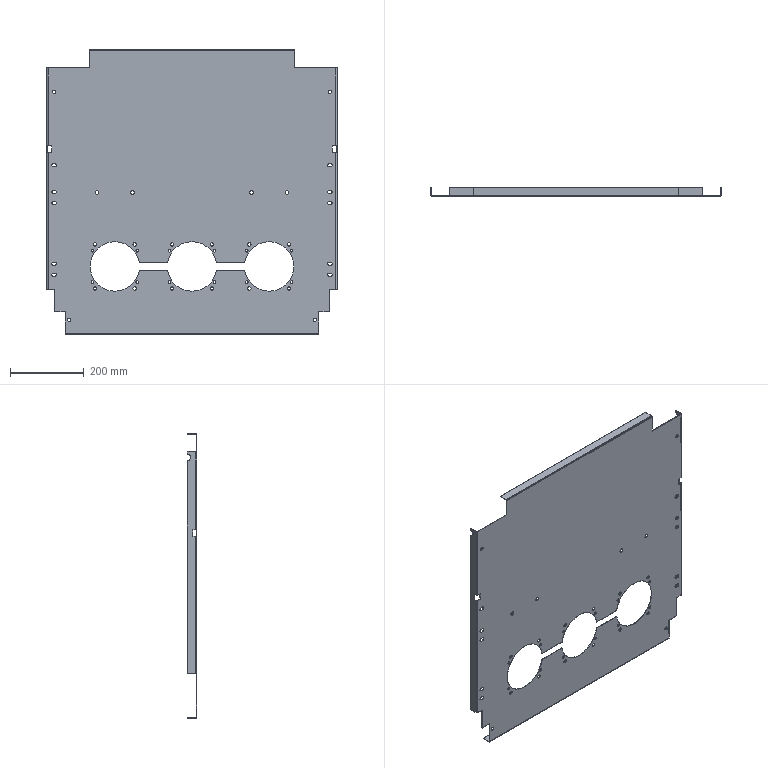Part | STEP file | 1 solid | 193 faces | box 789 x 25 x 775 mm | volume 895213 mm3 | cylinder 109 | plane 84 | commonest cylinder face diameters 9 x52 7 x24 135 x9 10 x8 3 x6 6 x6